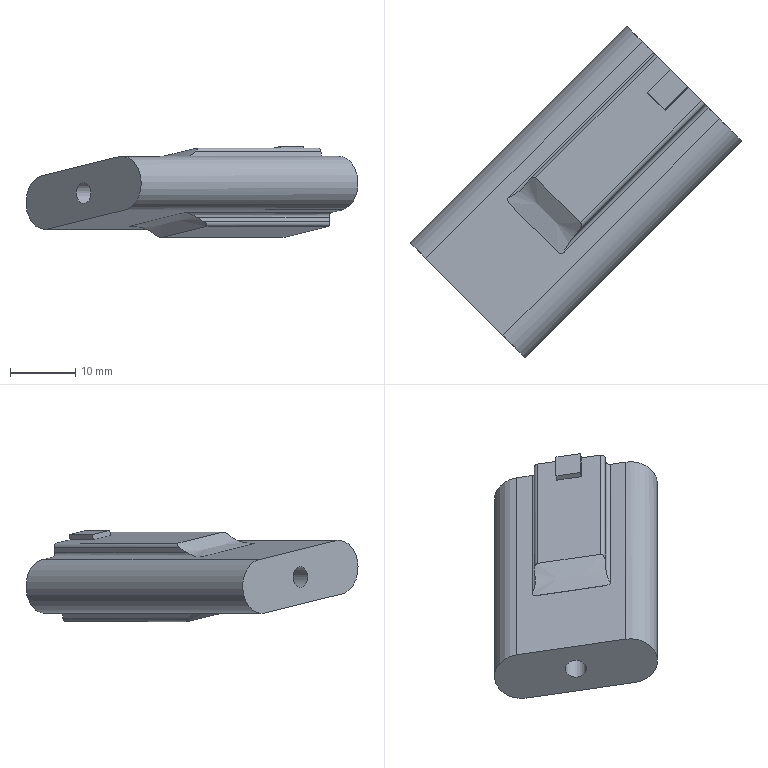Part | STEP file | gslz 2016.10.28-13_id350_x_t | 1 solid | 35 faces | box 50.906 x 50.906 x 13.989 mm | volume 9181 mm3 | spline 12 | plane 10 | cylinder 10 | other 3 | commonest cylinder face diameters 1.2 x8 3.2 x1 6.8 x1